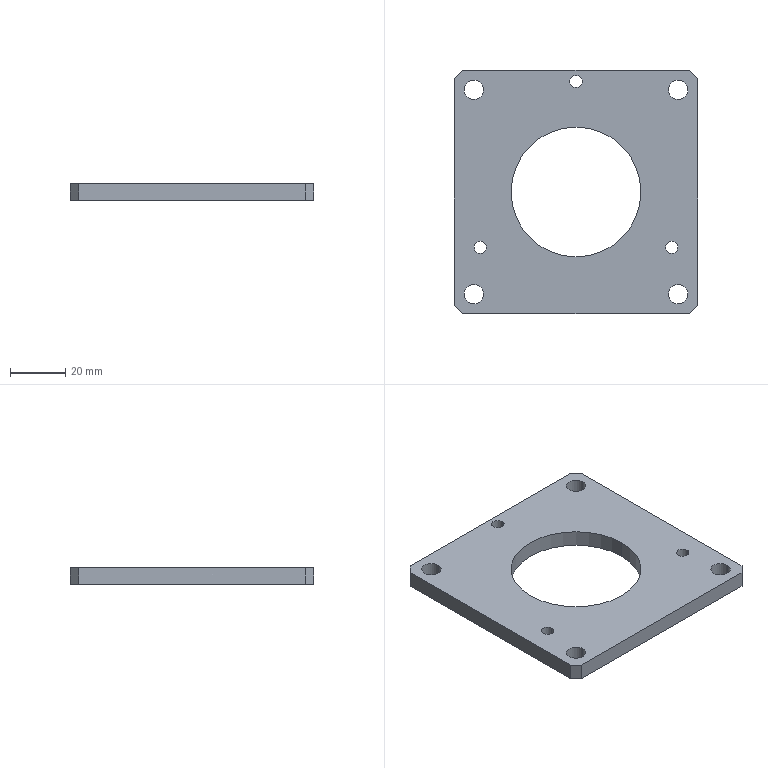Part | STEP file | MT-COMBO-119-S006 | 1 solid | 26 faces | box 88 x 88 x 6 mm | volume 34736 mm3 | cylinder 16 | plane 10 | commonest cylinder face diameters 7 x8 4.5 x6 47 x2
STEP:
#1=CARTESIAN_POINT('',(23.5,0.,6.));
#2=VERTEX_POINT('',#1);
#3=CARTESIAN_POINT('',(-23.5,0.,6.));
#4=VERTEX_POINT('',#3);
#5=CARTESIAN_POINT('',(0.,0.,6.));
#6=DIRECTION('',(0.,0.,1.));
#7=DIRECTION('',(-1.,0.,0.));
#8=AXIS2_PLACEMENT_3D('',#5,#6,#7);
#9=CIRCLE('',#8,23.5);
#10=EDGE_CURVE('',#2,#4,#9,.T.);
#11=ORIENTED_EDGE('',*,*,#10,.T.);
#12=CARTESIAN_POINT('',(-23.5,0.,0.));
#13=VERTEX_POINT('',#12);
#14=CARTESIAN_POINT('',(-23.5,0.,6.));
#15=DIRECTION('',(0.,0.,-1.));
#16=VECTOR('',#15,1000.);
#17=LINE('',#14,#16);
#18=EDGE_CURVE('',#4,#13,#17,.T.);
#19=ORIENTED_EDGE('',*,*,#18,.T.);
#20=CARTESIAN_POINT('',(23.5,0.,0.));
#21=VERTEX_POINT('',#20);
#22=CARTESIAN_POINT('',(0.,0.,0.));
#23=DIRECTION('',(0.,0.,1.));
#24=DIRECTION('',(-1.,0.,0.));
#25=AXIS2_PLACEMENT_3D('',#22,#23,#24);
#26=CIRCLE('',#25,23.5);
#27=EDGE_CURVE('',#21,#13,#26,.T.);
#28=ORIENTED_EDGE('',*,*,#27,.F.);
#29=CARTESIAN_POINT('',(23.5,0.,6.));
#30=DIRECTION('',(0.,0.,-1.));
#31=VECTOR('',#30,1000.);
#32=LINE('',#29,#31);
#33=EDGE_CURVE('',#2,#21,#32,.T.);
#34=ORIENTED_EDGE('',*,*,#33,.F.);
#35=EDGE_LOOP('',(#11,#19,#28,#34));
#36=FACE_OUTER_BOUND('',#35,.T.);
#37=CARTESIAN_POINT('',(0.,0.,6.));
#38=DIRECTION('',(0.,0.,-1.));
#39=DIRECTION('',(1.,0.,0.));
#40=AXIS2_PLACEMENT_3D('',#37,#38,#39);
#41=CYLINDRICAL_SURFACE('',#40,23.5);
#42=ADVANCED_FACE('',(#36),#41,.F.);
#43=CARTESIAN_POINT('',(-33.5,37.,6.));
#44=VERTEX_POINT('',#43);
#45=CARTESIAN_POINT('',(-40.5,37.,6.));
#46=VERTEX_POINT('',#45);
#47=CARTESIAN_POINT('',(-37.,37.,6.));
#48=DIRECTION('',(0.,0.,1.));
#49=DIRECTION('',(-1.,0.,0.));
#50=AXIS2_PLACEMENT_3D('',#47,#48,#49);
#51=CIRCLE('',#50,3.5);
#52=EDGE_CURVE('',#44,#46,#51,.T.);
#53=ORIENTED_EDGE('',*,*,#52,.T.);
#54=CARTESIAN_POINT('',(-40.5,37.,0.));
#55=VERTEX_POINT('',#54);
#56=CARTESIAN_POINT('',(-40.5,37.,6.));
#57=DIRECTION('',(0.,0.,-1.));
#58=VECTOR('',#57,1000.);
#59=LINE('',#56,#58);
#60=EDGE_CURVE('',#46,#55,#59,.T.);
#61=ORIENTED_EDGE('',*,*,#60,.T.);
#62=CARTESIAN_POINT('',(-33.5,37.,0.));
#63=VERTEX_POINT('',#62);
#64=CARTESIAN_POINT('',(-37.,37.,0.));
#65=DIRECTION('',(0.,0.,1.));
#66=DIRECTION('',(-1.,0.,0.));
#67=AXIS2_PLACEMENT_3D('',#64,#65,#66);
#68=CIRCLE('',#67,3.5);
#69=EDGE_CURVE('',#63,#55,#68,.T.);
#70=ORIENTED_EDGE('',*,*,#69,.F.);
#71=CARTESIAN_POINT('',(-33.5,37.,6.));
#72=DIRECTION('',(0.,0.,-1.));
#73=VECTOR('',#72,1000.);
#74=LINE('',#71,#73);
#75=EDGE_CURVE('',#44,#63,#74,.T.);
#76=ORIENTED_EDGE('',*,*,#75,.F.);
#77=EDGE_LOOP('',(#53,#61,#70,#76));
#78=FACE_OUTER_BOUND('',#77,.T.);
#79=CARTESIAN_POINT('',(-37.,37.,6.));
#80=DIRECTION('',(0.,0.,-1.));
#81=DIRECTION('',(1.,0.,0.));
#82=AXIS2_PLACEMENT_3D('',#79,#80,#81);
#83=CYLINDRICAL_SURFACE('',#82,3.5);
#84=ADVANCED_FACE('',(#78),#83,.F.);
#85=CARTESIAN_POINT('',(-33.5,-37.,6.));
#86=VERTEX_POINT('',#85);
#87=CARTESIAN_POINT('',(-40.5,-37.,6.));
#88=VERTEX_POINT('',#87);
#89=CARTESIAN_POINT('',(-37.,-37.,6.));
#90=DIRECTION('',(0.,0.,1.));
#91=DIRECTION('',(-1.,0.,0.));
#92=AXIS2_PLACEMENT_3D('',#89,#90,#91);
#93=CIRCLE('',#92,3.5);
#94=EDGE_CURVE('',#86,#88,#93,.T.);
#95=ORIENTED_EDGE('',*,*,#94,.T.);
#96=CARTESIAN_POINT('',(-40.5,-37.,0.));
#97=VERTEX_POINT('',#96);
#98=CARTESIAN_POINT('',(-40.5,-37.,6.));
#99=DIRECTION('',(0.,0.,-1.));
#100=VECTOR('',#99,1000.);
#101=LINE('',#98,#100);
#102=EDGE_CURVE('',#88,#97,#101,.T.);
#103=ORIENTED_EDGE('',*,*,#102,.T.);
#104=CARTESIAN_POINT('',(-33.5,-37.,0.));
#105=VERTEX_POINT('',#104);
#106=CARTESIAN_POINT('',(-37.,-37.,0.));
#107=DIRECTION('',(0.,0.,1.));
#108=DIRECTION('',(-1.,0.,0.));
#109=AXIS2_PLACEMENT_3D('',#106,#107,#108);
#110=CIRCLE('',#109,3.5);
#111=EDGE_CURVE('',#105,#97,#110,.T.);
#112=ORIENTED_EDGE('',*,*,#111,.F.);
#113=CARTESIAN_POINT('',(-33.5,-37.,6.));
#114=DIRECTION('',(0.,0.,-1.));
#115=VECTOR('',#114,1000.);
#116=LINE('',#113,#115);
#117=EDGE_CURVE('',#86,#105,#116,.T.);
#118=ORIENTED_EDGE('',*,*,#117,.F.);
#119=EDGE_LOOP('',(#95,#103,#112,#118));
#120=FACE_OUTER_BOUND('',#119,.T.);
#121=CARTESIAN_POINT('',(-37.,-37.,6.));
#122=DIRECTION('',(0.,0.,-1.));
#123=DIRECTION('',(1.,0.,0.));
#124=AXIS2_PLACEMENT_3D('',#121,#122,#123);
#125=CYLINDRICAL_SURFACE('',#124,3.5);
#126=ADVANCED_FACE('',(#120),#125,.F.);
#127=CARTESIAN_POINT('',(40.5,-37.,6.));
#128=VERTEX_POINT('',#127);
#129=CARTESIAN_POINT('',(33.5,-37.,6.));
#130=VERTEX_POINT('',#129);
#131=CARTESIAN_POINT('',(37.,-37.,6.));
#132=DIRECTION('',(0.,0.,1.));
#133=DIRECTION('',(-1.,0.,0.));
#134=AXIS2_PLACEMENT_3D('',#131,#132,#133);
#135=CIRCLE('',#134,3.5);
#136=EDGE_CURVE('',#128,#130,#135,.T.);
#137=ORIENTED_EDGE('',*,*,#136,.T.);
#138=CARTESIAN_POINT('',(33.5,-37.,0.));
#139=VERTEX_POINT('',#138);
#140=CARTESIAN_POINT('',(33.5,-37.,6.));
#141=DIRECTION('',(0.,0.,-1.));
#142=VECTOR('',#141,1000.);
#143=LINE('',#140,#142);
#144=EDGE_CURVE('',#130,#139,#143,.T.);
#145=ORIENTED_EDGE('',*,*,#144,.T.);
#146=CARTESIAN_POINT('',(40.5,-37.,0.));
#147=VERTEX_POINT('',#146);
#148=CARTESIAN_POINT('',(37.,-37.,0.));
#149=DIRECTION('',(0.,0.,1.));
#150=DIRECTION('',(-1.,0.,0.));
#151=AXIS2_PLACEMENT_3D('',#148,#149,#150);
#152=CIRCLE('',#151,3.5);
#153=EDGE_CURVE('',#147,#139,#152,.T.);
#154=ORIENTED_EDGE('',*,*,#153,.F.);
#155=CARTESIAN_POINT('',(40.5,-37.,6.));
#156=DIRECTION('',(0.,0.,-1.));
#157=VECTOR('',#156,1000.);
#158=LINE('',#155,#157);
#159=EDGE_CURVE('',#128,#147,#158,.T.);
#160=ORIENTED_EDGE('',*,*,#159,.F.);
#161=EDGE_LOOP('',(#137,#145,#154,#160));
#162=FACE_OUTER_BOUND('',#161,.T.);
#163=CARTESIAN_POINT('',(37.,-37.,6.));
#164=DIRECTION('',(0.,0.,-1.));
#165=DIRECTION('',(1.,0.,0.));
#166=AXIS2_PLACEMENT_3D('',#163,#164,#165);
#167=CYLINDRICAL_SURFACE('',#166,3.5);
#168=ADVANCED_FACE('',(#162),#167,.F.);
#169=CARTESIAN_POINT('',(40.5,37.,6.));
#170=VERTEX_POINT('',#169);
#171=CARTESIAN_POINT('',(33.5,37.,6.));
#172=VERTEX_POINT('',#171);
#173=CARTESIAN_POINT('',(37.,37.,6.));
#174=DIRECTION('',(0.,0.,1.));
#175=DIRECTION('',(-1.,0.,0.));
#176=AXIS2_PLACEMENT_3D('',#173,#174,#175);
#177=CIRCLE('',#176,3.5);
#178=EDGE_CURVE('',#170,#172,#177,.T.);
#179=ORIENTED_EDGE('',*,*,#178,.T.);
#180=CARTESIAN_POINT('',(33.5,37.,0.));
#181=VERTEX_POINT('',#180);
#182=CARTESIAN_POINT('',(33.5,37.,6.));
#183=DIRECTION('',(0.,0.,-1.));
#184=VECTOR('',#183,1000.);
#185=LINE('',#182,#184);
#186=EDGE_CURVE('',#172,#181,#185,.T.);
#187=ORIENTED_EDGE('',*,*,#186,.T.);
#188=CARTESIAN_POINT('',(40.5,37.,0.));
#189=VERTEX_POINT('',#188);
#190=CARTESIAN_POINT('',(37.,37.,0.));
#191=DIRECTION('',(0.,0.,1.));
#192=DIRECTION('',(-1.,0.,0.));
#193=AXIS2_PLACEMENT_3D('',#190,#191,#192);
#194=CIRCLE('',#193,3.5);
#195=EDGE_CURVE('',#189,#181,#194,.T.);
#196=ORIENTED_EDGE('',*,*,#195,.F.);
#197=CARTESIAN_POINT('',(40.5,37.,6.));
#198=DIRECTION('',(0.,0.,-1.));
#199=VECTOR('',#198,1000.);
#200=LINE('',#197,#199);
#201=EDGE_CURVE('',#170,#189,#200,.T.);
#202=ORIENTED_EDGE('',*,*,#201,.F.);
#203=EDGE_LOOP('',(#179,#187,#196,#202));
#204=FACE_OUTER_BOUND('',#203,.T.);
#205=CARTESIAN_POINT('',(37.,37.,6.));
#206=DIRECTION('',(0.,0.,-1.));
#207=DIRECTION('',(1.,0.,0.));
#208=AXIS2_PLACEMENT_3D('',#205,#206,#207);
#209=CYLINDRICAL_SURFACE('',#208,3.5);
#210=ADVANCED_FACE('',(#204),#209,.F.);
#211=CARTESIAN_POINT('',(2.25,40.,6.));
#212=VERTEX_POINT('',#211);
#213=CARTESIAN_POINT('',(-2.25,40.,6.));
#214=VERTEX_POINT('',#213);
#215=CARTESIAN_POINT('',(0.,40.,6.));
#216=DIRECTION('',(0.,0.,1.));
#217=DIRECTION('',(-1.,0.,0.));
#218=AXIS2_PLACEMENT_3D('',#215,#216,#217);
#219=CIRCLE('',#218,2.25);
#220=EDGE_CURVE('',#212,#214,#219,.T.);
#221=ORIENTED_EDGE('',*,*,#220,.T.);
#222=CARTESIAN_POINT('',(-2.25,40.,0.));
#223=VERTEX_POINT('',#222);
#224=CARTESIAN_POINT('',(-2.25,40.,6.));
#225=DIRECTION('',(0.,0.,-1.));
#226=VECTOR('',#225,1000.);
#227=LINE('',#224,#226);
#228=EDGE_CURVE('',#214,#223,#227,.T.);
#229=ORIENTED_EDGE('',*,*,#228,.T.);
#230=CARTESIAN_POINT('',(2.25,40.,0.));
#231=VERTEX_POINT('',#230);
#232=CARTESIAN_POINT('',(0.,40.,0.));
#233=DIRECTION('',(0.,0.,1.));
#234=DIRECTION('',(-1.,0.,0.));
#235=AXIS2_PLACEMENT_3D('',#232,#233,#234);
#236=CIRCLE('',#235,2.25);
#237=EDGE_CURVE('',#231,#223,#236,.T.);
#238=ORIENTED_EDGE('',*,*,#237,.F.);
#239=CARTESIAN_POINT('',(2.25,40.,6.));
#240=DIRECTION('',(0.,0.,-1.));
#241=VECTOR('',#240,1000.);
#242=LINE('',#239,#241);
#243=EDGE_CURVE('',#212,#231,#242,.T.);
#244=ORIENTED_EDGE('',*,*,#243,.F.);
#245=EDGE_LOOP('',(#221,#229,#238,#244));
#246=FACE_OUTER_BOUND('',#245,.T.);
#247=CARTESIAN_POINT('',(0.,40.,6.));
#248=DIRECTION('',(0.,0.,-1.));
#249=DIRECTION('',(1.,0.,0.));
#250=AXIS2_PLACEMENT_3D('',#247,#248,#249);
#251=CYLINDRICAL_SURFACE('',#250,2.25);
#252=ADVANCED_FACE('',(#246),#251,.F.);
#253=CARTESIAN_POINT('',(-32.391,-20.,6.));
#254=VERTEX_POINT('',#253);
#255=CARTESIAN_POINT('',(-36.891,-20.,6.));
#256=VERTEX_POINT('',#255);
#257=CARTESIAN_POINT('',(-34.641,-20.,6.));
#258=DIRECTION('',(0.,0.,1.));
#259=DIRECTION('',(-1.,0.,0.));
#260=AXIS2_PLACEMENT_3D('',#257,#258,#259);
#261=CIRCLE('',#260,2.25);
#262=EDGE_CURVE('',#254,#256,#261,.T.);
#263=ORIENTED_EDGE('',*,*,#262,.T.);
#264=CARTESIAN_POINT('',(-36.891,-20.,0.));
#265=VERTEX_POINT('',#264);
#266=CARTESIAN_POINT('',(-36.891,-20.,6.));
#267=DIRECTION('',(0.,0.,-1.));
#268=VECTOR('',#267,1000.);
#269=LINE('',#266,#268);
#270=EDGE_CURVE('',#256,#265,#269,.T.);
#271=ORIENTED_EDGE('',*,*,#270,.T.);
#272=CARTESIAN_POINT('',(-32.391,-20.,0.));
#273=VERTEX_POINT('',#272);
#274=CARTESIAN_POINT('',(-34.641,-20.,0.));
#275=DIRECTION('',(0.,0.,1.));
#276=DIRECTION('',(-1.,0.,0.));
#277=AXIS2_PLACEMENT_3D('',#274,#275,#276);
#278=CIRCLE('',#277,2.25);
#279=EDGE_CURVE('',#273,#265,#278,.T.);
#280=ORIENTED_EDGE('',*,*,#279,.F.);
#281=CARTESIAN_POINT('',(-32.391,-20.,6.));
#282=DIRECTION('',(0.,0.,-1.));
#283=VECTOR('',#282,1000.);
#284=LINE('',#281,#283);
#285=EDGE_CURVE('',#254,#273,#284,.T.);
#286=ORIENTED_EDGE('',*,*,#285,.F.);
#287=EDGE_LOOP('',(#263,#271,#280,#286));
#288=FACE_OUTER_BOUND('',#287,.T.);
#289=CARTESIAN_POINT('',(-34.641,-20.,6.));
#290=DIRECTION('',(0.,0.,-1.));
#291=DIRECTION('',(1.,0.,0.));
#292=AXIS2_PLACEMENT_3D('',#289,#290,#291);
#293=CYLINDRICAL_SURFACE('',#292,2.25);
#294=ADVANCED_FACE('',(#288),#293,.F.);
#295=CARTESIAN_POINT('',(36.891,-20.,6.));
#296=VERTEX_POINT('',#295);
#297=CARTESIAN_POINT('',(32.391,-20.,6.));
#298=VERTEX_POINT('',#297);
#299=CARTESIAN_POINT('',(34.641,-20.,6.));
#300=DIRECTION('',(0.,0.,1.));
#301=DIRECTION('',(-1.,0.,0.));
#302=AXIS2_PLACEMENT_3D('',#299,#300,#301);
#303=CIRCLE('',#302,2.25);
#304=EDGE_CURVE('',#296,#298,#303,.T.);
#305=ORIENTED_EDGE('',*,*,#304,.T.);
#306=CARTESIAN_POINT('',(32.391,-20.,0.));
#307=VERTEX_POINT('',#306);
#308=CARTESIAN_POINT('',(32.391,-20.,6.));
#309=DIRECTION('',(0.,0.,-1.));
#310=VECTOR('',#309,1000.);
#311=LINE('',#308,#310);
#312=EDGE_CURVE('',#298,#307,#311,.T.);
#313=ORIENTED_EDGE('',*,*,#312,.T.);
#314=CARTESIAN_POINT('',(36.891,-20.,0.));
#315=VERTEX_POINT('',#314);
#316=CARTESIAN_POINT('',(34.641,-20.,0.));
#317=DIRECTION('',(0.,0.,1.));
#318=DIRECTION('',(-1.,0.,0.));
#319=AXIS2_PLACEMENT_3D('',#316,#317,#318);
#320=CIRCLE('',#319,2.25);
#321=EDGE_CURVE('',#315,#307,#320,.T.);
#322=ORIENTED_EDGE('',*,*,#321,.F.);
#323=CARTESIAN_POINT('',(36.891,-20.,6.));
#324=DIRECTION('',(0.,0.,-1.));
#325=VECTOR('',#324,1000.);
#326=LINE('',#323,#325);
#327=EDGE_CURVE('',#296,#315,#326,.T.);
#328=ORIENTED_EDGE('',*,*,#327,.F.);
#329=EDGE_LOOP('',(#305,#313,#322,#328));
#330=FACE_OUTER_BOUND('',#329,.T.);
#331=CARTESIAN_POINT('',(34.641,-20.,6.));
#332=DIRECTION('',(0.,0.,-1.));
#333=DIRECTION('',(1.,0.,0.));
#334=AXIS2_PLACEMENT_3D('',#331,#332,#333);
#335=CYLINDRICAL_SURFACE('',#334,2.25);
#336=ADVANCED_FACE('',(#330),#335,.F.);
#337=CARTESIAN_POINT('',(41.,44.,6.));
#338=VERTEX_POINT('',#337);
#339=CARTESIAN_POINT('',(-41.,44.,6.));
#340=VERTEX_POINT('',#339);
#341=CARTESIAN_POINT('',(44.,44.,6.));
#342=DIRECTION('',(-1.,0.,0.));
#343=VECTOR('',#342,1000.);
#344=LINE('',#341,#343);
#345=EDGE_CURVE('',#338,#340,#344,.T.);
#346=ORIENTED_EDGE('',*,*,#345,.F.);
#347=CARTESIAN_POINT('',(41.,44.,0.));
#348=VERTEX_POINT('',#347);
#349=CARTESIAN_POINT('',(41.,44.,6.));
#350=DIRECTION('',(0.,0.,1.));
#351=VECTOR('',#350,1000.);
#352=LINE('',#349,#351);
#353=EDGE_CURVE('',#348,#338,#352,.T.);
#354=ORIENTED_EDGE('',*,*,#353,.F.);
#355=CARTESIAN_POINT('',(-41.,44.,0.));
#356=VERTEX_POINT('',#355);
#357=CARTESIAN_POINT('',(44.,44.,0.));
#358=DIRECTION('',(-1.,0.,0.));
#359=VECTOR('',#358,1000.);
#360=LINE('',#357,#359);
#361=EDGE_CURVE('',#348,#356,#360,.T.);
#362=ORIENTED_EDGE('',*,*,#361,.T.);
#363=CARTESIAN_POINT('',(-41.,44.,6.));
#364=DIRECTION('',(0.,0.,-1.));
#365=VECTOR('',#364,1000.);
#366=LINE('',#363,#365);
#367=EDGE_CURVE('',#340,#356,#366,.T.);
#368=ORIENTED_EDGE('',*,*,#367,.F.);
#369=EDGE_LOOP('',(#346,#354,#362,#368));
#370=FACE_OUTER_BOUND('',#369,.T.);
#371=CARTESIAN_POINT('',(44.,44.,6.));
#372=DIRECTION('',(0.,1.,0.));
#373=DIRECTION('',(0.,0.,-1.));
#374=AXIS2_PLACEMENT_3D('',#371,#372,#373);
#375=PLANE('',#374);
#376=ADVANCED_FACE('',(#370),#375,.T.);
#377=CARTESIAN_POINT('',(44.,-41.,0.));
#378=VERTEX_POINT('',#377);
#379=CARTESIAN_POINT('',(44.,41.,0.));
#380=VERTEX_POINT('',#379);
#381=CARTESIAN_POINT('',(44.,-44.,0.));
#382=DIRECTION('',(0.,1.,0.));
#383=VECTOR('',#382,1000.);
#384=LINE('',#381,#383);
#385=EDGE_CURVE('',#378,#380,#384,.T.);
#386=ORIENTED_EDGE('',*,*,#385,.T.);
#387=CARTESIAN_POINT('',(44.,41.,6.));
#388=VERTEX_POINT('',#387);
#389=CARTESIAN_POINT('',(44.,41.,6.));
#390=DIRECTION('',(0.,0.,-1.));
#391=VECTOR('',#390,1000.);
#392=LINE('',#389,#391);
#393=EDGE_CURVE('',#388,#380,#392,.T.);
#394=ORIENTED_EDGE('',*,*,#393,.F.);
#395=CARTESIAN_POINT('',(44.,-41.,6.));
#396=VERTEX_POINT('',#395);
#397=CARTESIAN_POINT('',(44.,-44.,6.));
#398=DIRECTION('',(0.,1.,0.));
#399=VECTOR('',#398,1000.);
#400=LINE('',#397,#399);
#401=EDGE_CURVE('',#396,#388,#400,.T.);
#402=ORIENTED_EDGE('',*,*,#401,.F.);
#403=CARTESIAN_POINT('',(44.,-41.,6.));
#404=DIRECTION('',(0.,0.,1.));
#405=VECTOR('',#404,1000.);
#406=LINE('',#403,#405);
#407=EDGE_CURVE('',#378,#396,#406,.T.);
#408=ORIENTED_EDGE('',*,*,#407,.F.);
#409=EDGE_LOOP('',(#386,#394,#402,#408));
#410=FACE_OUTER_BOUND('',#409,.T.);
#411=CARTESIAN_POINT('',(44.,-44.,6.));
#412=DIRECTION('',(1.,0.,0.));
#413=DIRECTION('',(0.,1.,0.));
#414=AXIS2_PLACEMENT_3D('',#411,#412,#413);
#415=PLANE('',#414);
#416=ADVANCED_FACE('',(#410),#415,.T.);
#417=CARTESIAN_POINT('',(-41.,-44.,0.));
#418=VERTEX_POINT('',#417);
#419=CARTESIAN_POINT('',(41.,-44.,0.));
#420=VERTEX_POINT('',#419);
#421=CARTESIAN_POINT('',(-44.,-44.,0.));
#422=DIRECTION('',(1.,0.,0.));
#423=VECTOR('',#422,1000.);
#424=LINE('',#421,#423);
#425=EDGE_CURVE('',#418,#420,#424,.T.);
#426=ORIENTED_EDGE('',*,*,#425,.T.);
#427=CARTESIAN_POINT('',(41.,-44.,6.));
#428=VERTEX_POINT('',#427);
#429=CARTESIAN_POINT('',(41.,-44.,6.));
#430=DIRECTION('',(0.,0.,-1.));
#431=VECTOR('',#430,1000.);
#432=LINE('',#429,#431);
#433=EDGE_CURVE('',#428,#420,#432,.T.);
#434=ORIENTED_EDGE('',*,*,#433,.F.);
#435=CARTESIAN_POINT('',(-41.,-44.,6.));
#436=VERTEX_POINT('',#435);
#437=CARTESIAN_POINT('',(-44.,-44.,6.));
#438=DIRECTION('',(1.,0.,0.));
#439=VECTOR('',#438,1000.);
#440=LINE('',#437,#439);
#441=EDGE_CURVE('',#436,#428,#440,.T.);
#442=ORIENTED_EDGE('',*,*,#441,.F.);
#443=CARTESIAN_POINT('',(-41.,-44.,6.));
#444=DIRECTION('',(0.,0.,1.));
#445=VECTOR('',#444,1000.);
#446=LINE('',#443,#445);
#447=EDGE_CURVE('',#418,#436,#446,.T.);
#448=ORIENTED_EDGE('',*,*,#447,.F.);
#449=EDGE_LOOP('',(#426,#434,#442,#448));
#450=FACE_OUTER_BOUND('',#449,.T.);
#451=CARTESIAN_POINT('',(-44.,-44.,6.));
#452=DIRECTION('',(0.,-1.,0.));
#453=DIRECTION('',(0.,0.,1.));
#454=AXIS2_PLACEMENT_3D('',#451,#452,#453);
#455=PLANE('',#454);
#456=ADVANCED_FACE('',(#450),#455,.T.);
#457=CARTESIAN_POINT('',(-44.,41.,6.));
#458=VERTEX_POINT('',#457);
#459=CARTESIAN_POINT('',(-44.,-41.,6.));
#460=VERTEX_POINT('',#459);
#461=CARTESIAN_POINT('',(-44.,44.,6.));
#462=DIRECTION('',(0.,-1.,0.));
#463=VECTOR('',#462,1000.);
#464=LINE('',#461,#463);
#465=EDGE_CURVE('',#458,#460,#464,.T.);
#466=ORIENTED_EDGE('',*,*,#465,.F.);
#467=CARTESIAN_POINT('',(-44.,41.,0.));
#468=VERTEX_POINT('',#467);
#469=CARTESIAN_POINT('',(-44.,41.,6.));
#470=DIRECTION('',(0.,0.,1.));
#471=VECTOR('',#470,1000.);
#472=LINE('',#469,#471);
#473=EDGE_CURVE('',#468,#458,#472,.T.);
#474=ORIENTED_EDGE('',*,*,#473,.F.);
#475=CARTESIAN_POINT('',(-44.,-41.,0.));
#476=VERTEX_POINT('',#475);
#477=CARTESIAN_POINT('',(-44.,44.,0.));
#478=DIRECTION('',(0.,-1.,0.));
#479=VECTOR('',#478,1000.);
#480=LINE('',#477,#479);
#481=EDGE_CURVE('',#468,#476,#480,.T.);
#482=ORIENTED_EDGE('',*,*,#481,.T.);
#483=CARTESIAN_POINT('',(-44.,-41.,6.));
#484=DIRECTION('',(0.,0.,-1.));
#485=VECTOR('',#484,1000.);
#486=LINE('',#483,#485);
#487=EDGE_CURVE('',#460,#476,#486,.T.);
#488=ORIENTED_EDGE('',*,*,#487,.F.);
#489=EDGE_LOOP('',(#466,#474,#482,#488));
#490=FACE_OUTER_BOUND('',#489,.T.);
#491=CARTESIAN_POINT('',(-44.,44.,6.));
#492=DIRECTION('',(-1.,0.,0.));
#493=DIRECTION('',(0.,-1.,0.));
#494=AXIS2_PLACEMENT_3D('',#491,#492,#493);
#495=PLANE('',#494);
#496=ADVANCED_FACE('',(#490),#495,.T.);
#497=ORIENTED_EDGE('',*,*,#10,.F.);
#498=CARTESIAN_POINT('',(0.,0.,6.));
#499=DIRECTION('',(0.,0.,1.));
#500=DIRECTION('',(-1.,0.,0.));
#501=AXIS2_PLACEMENT_3D('',#498,#499,#500);
#502=CIRCLE('',#501,23.5);
#503=EDGE_CURVE('',#4,#2,#502,.T.);
#504=ORIENTED_EDGE('',*,*,#503,.F.);
#505=EDGE_LOOP('',(#497,#504));
#506=FACE_BOUND('',#505,.T.);
#507=ORIENTED_EDGE('',*,*,#52,.F.);
#508=CARTESIAN_POINT('',(-37.,37.,6.));
#509=DIRECTION('',(0.,0.,1.));
#510=DIRECTION('',(-1.,0.,0.));
#511=AXIS2_PLACEMENT_3D('',#508,#509,#510);
#512=CIRCLE('',#511,3.5);
#513=EDGE_CURVE('',#46,#44,#512,.T.);
#514=ORIENTED_EDGE('',*,*,#513,.F.);
#515=EDGE_LOOP('',(#507,#514));
#516=FACE_BOUND('',#515,.T.);
#517=ORIENTED_EDGE('',*,*,#94,.F.);
#518=CARTESIAN_POINT('',(-37.,-37.,6.));
#519=DIRECTION('',(0.,0.,1.));
#520=DIRECTION('',(-1.,0.,0.));
#521=AXIS2_PLACEMENT_3D('',#518,#519,#520);
#522=CIRCLE('',#521,3.5);
#523=EDGE_CURVE('',#88,#86,#522,.T.);
#524=ORIENTED_EDGE('',*,*,#523,.F.);
#525=EDGE_LOOP('',(#517,#524));
#526=FACE_BOUND('',#525,.T.);
#527=ORIENTED_EDGE('',*,*,#136,.F.);
#528=CARTESIAN_POINT('',(37.,-37.,6.));
#529=DIRECTION('',(0.,0.,1.));
#530=DIRECTION('',(-1.,0.,0.));
#531=AXIS2_PLACEMENT_3D('',#528,#529,#530);
#532=CIRCLE('',#531,3.5);
#533=EDGE_CURVE('',#130,#128,#532,.T.);
#534=ORIENTED_EDGE('',*,*,#533,.F.);
#535=EDGE_LOOP('',(#527,#534));
#536=FACE_BOUND('',#535,.T.);
#537=ORIENTED_EDGE('',*,*,#178,.F.);
#538=CARTESIAN_POINT('',(37.,37.,6.));
#539=DIRECTION('',(0.,0.,1.));
#540=DIRECTION('',(-1.,0.,0.));
#541=AXIS2_PLACEMENT_3D('',#538,#539,#540);
#542=CIRCLE('',#541,3.5);
#543=EDGE_CURVE('',#172,#170,#542,.T.);
#544=ORIENTED_EDGE('',*,*,#543,.F.);
#545=EDGE_LOOP('',(#537,#544));
#546=FACE_BOUND('',#545,.T.);
#547=ORIENTED_EDGE('',*,*,#220,.F.);
#548=CARTESIAN_POINT('',(0.,40.,6.));
#549=DIRECTION('',(0.,0.,1.));
#550=DIRECTION('',(-1.,0.,0.));
#551=AXIS2_PLACEMENT_3D('',#548,#549,#550);
#552=CIRCLE('',#551,2.25);
#553=EDGE_CURVE('',#214,#212,#552,.T.);
#554=ORIENTED_EDGE('',*,*,#553,.F.);
#555=EDGE_LOOP('',(#547,#554));
#556=FACE_BOUND('',#555,.T.);
#557=ORIENTED_EDGE('',*,*,#262,.F.);
#558=CARTESIAN_POINT('',(-34.641,-20.,6.));
#559=DIRECTION('',(0.,0.,1.));
#560=DIRECTION('',(-1.,0.,0.));
#561=AXIS2_PLACEMENT_3D('',#558,#559,#560);
#562=CIRCLE('',#561,2.25);
#563=EDGE_CURVE('',#256,#254,#562,.T.);
#564=ORIENTED_EDGE('',*,*,#563,.F.);
#565=EDGE_LOOP('',(#557,#564));
#566=FACE_BOUND('',#565,.T.);
#567=ORIENTED_EDGE('',*,*,#304,.F.);
#568=CARTESIAN_POINT('',(34.641,-20.,6.));
#569=DIRECTION('',(0.,0.,1.));
#570=DIRECTION('',(-1.,0.,0.));
#571=AXIS2_PLACEMENT_3D('',#568,#569,#570);
#572=CIRCLE('',#571,2.25);
#573=EDGE_CURVE('',#298,#296,#572,.T.);
#574=ORIENTED_EDGE('',*,*,#573,.F.);
#575=EDGE_LOOP('',(#567,#574));
#576=FACE_BOUND('',#575,.T.);
#577=ORIENTED_EDGE('',*,*,#441,.T.);
#578=CARTESIAN_POINT('',(41.,-44.,6.));
#579=DIRECTION('',(-0.7071,-0.7071,0.));
#580=VECTOR('',#579,1000.);
#581=LINE('',#578,#580);
#582=EDGE_CURVE('',#396,#428,#581,.T.);
#583=ORIENTED_EDGE('',*,*,#582,.F.);
#584=ORIENTED_EDGE('',*,*,#401,.T.);
#585=CARTESIAN_POINT('',(44.,41.,6.));
#586=DIRECTION('',(0.7071,-0.7071,0.));
#587=VECTOR('',#586,1000.);
#588=LINE('',#585,#587);
#589=EDGE_CURVE('',#338,#388,#588,.T.);
#590=ORIENTED_EDGE('',*,*,#589,.F.);
#591=ORIENTED_EDGE('',*,*,#345,.T.);
#592=CARTESIAN_POINT('',(-41.,44.,6.));
#593=DIRECTION('',(0.7071,0.7071,0.));
#594=VECTOR('',#593,1000.);
#595=LINE('',#592,#594);
#596=EDGE_CURVE('',#458,#340,#595,.T.);
#597=ORIENTED_EDGE('',*,*,#596,.F.);
#598=ORIENTED_EDGE('',*,*,#465,.T.);
#599=CARTESIAN_POINT('',(-44.,-41.,6.));
#600=DIRECTION('',(-0.7071,0.7071,0.));
#601=VECTOR('',#600,1000.);
#602=LINE('',#599,#601);
#603=EDGE_CURVE('',#436,#460,#602,.T.);
#604=ORIENTED_EDGE('',*,*,#603,.F.);
#605=EDGE_LOOP('',(#577,#583,#584,#590,#591,#597,#598,#604));
#606=FACE_OUTER_BOUND('',#605,.T.);
#607=CARTESIAN_POINT('',(0.,0.,6.));
#608=DIRECTION('',(0.,0.,-1.));
#609=DIRECTION('',(1.,0.,0.));
#610=AXIS2_PLACEMENT_3D('',#607,#608,#609);
#611=PLANE('',#610);
#612=ADVANCED_FACE('',(#506,#516,#526,#536,#546,#556,#566,#576,#606),#611,.F.);
#613=ORIENTED_EDGE('',*,*,#27,.T.);
#614=CARTESIAN_POINT('',(0.,0.,0.));
#615=DIRECTION('',(0.,0.,1.));
#616=DIRECTION('',(-1.,0.,0.));
#617=AXIS2_PLACEMENT_3D('',#614,#615,#616);
#618=CIRCLE('',#617,23.5);
#619=EDGE_CURVE('',#13,#21,#618,.T.);
#620=ORIENTED_EDGE('',*,*,#619,.T.);
#621=EDGE_LOOP('',(#613,#620));
#622=FACE_BOUND('',#621,.T.);
#623=ORIENTED_EDGE('',*,*,#69,.T.);
#624=CARTESIAN_POINT('',(-37.,37.,0.));
#625=DIRECTION('',(0.,0.,1.));
#626=DIRECTION('',(-1.,0.,0.));
#627=AXIS2_PLACEMENT_3D('',#624,#625,#626);
#628=CIRCLE('',#627,3.5);
#629=EDGE_CURVE('',#55,#63,#628,.T.);
#630=ORIENTED_EDGE('',*,*,#629,.T.);
#631=EDGE_LOOP('',(#623,#630));
#632=FACE_BOUND('',#631,.T.);
#633=ORIENTED_EDGE('',*,*,#111,.T.);
#634=CARTESIAN_POINT('',(-37.,-37.,0.));
#635=DIRECTION('',(0.,0.,1.));
#636=DIRECTION('',(-1.,0.,0.));
#637=AXIS2_PLACEMENT_3D('',#634,#635,#636);
#638=CIRCLE('',#637,3.5);
#639=EDGE_CURVE('',#97,#105,#638,.T.);
#640=ORIENTED_EDGE('',*,*,#639,.T.);
#641=EDGE_LOOP('',(#633,#640));
#642=FACE_BOUND('',#641,.T.);
#643=ORIENTED_EDGE('',*,*,#153,.T.);
#644=CARTESIAN_POINT('',(37.,-37.,0.));
#645=DIRECTION('',(0.,0.,1.));
#646=DIRECTION('',(-1.,0.,0.));
#647=AXIS2_PLACEMENT_3D('',#644,#645,#646);
#648=CIRCLE('',#647,3.5);
#649=EDGE_CURVE('',#139,#147,#648,.T.);
#650=ORIENTED_EDGE('',*,*,#649,.T.);
#651=EDGE_LOOP('',(#643,#650));
#652=FACE_BOUND('',#651,.T.);
#653=ORIENTED_EDGE('',*,*,#195,.T.);
#654=CARTESIAN_POINT('',(37.,37.,0.));
#655=DIRECTION('',(0.,0.,1.));
#656=DIRECTION('',(-1.,0.,0.));
#657=AXIS2_PLACEMENT_3D('',#654,#655,#656);
#658=CIRCLE('',#657,3.5);
#659=EDGE_CURVE('',#181,#189,#658,.T.);
#660=ORIENTED_EDGE('',*,*,#659,.T.);
#661=EDGE_LOOP('',(#653,#660));
#662=FACE_BOUND('',#661,.T.);
#663=ORIENTED_EDGE('',*,*,#237,.T.);
#664=CARTESIAN_POINT('',(0.,40.,0.));
#665=DIRECTION('',(0.,0.,1.));
#666=DIRECTION('',(-1.,0.,0.));
#667=AXIS2_PLACEMENT_3D('',#664,#665,#666);
#668=CIRCLE('',#667,2.25);
#669=EDGE_CURVE('',#223,#231,#668,.T.);
#670=ORIENTED_EDGE('',*,*,#669,.T.);
#671=EDGE_LOOP('',(#663,#670));
#672=FACE_BOUND('',#671,.T.);
#673=ORIENTED_EDGE('',*,*,#279,.T.);
#674=CARTESIAN_POINT('',(-34.641,-20.,0.));
#675=DIRECTION('',(0.,0.,1.));
#676=DIRECTION('',(-1.,0.,0.));
#677=AXIS2_PLACEMENT_3D('',#674,#675,#676);
#678=CIRCLE('',#677,2.25);
#679=EDGE_CURVE('',#265,#273,#678,.T.);
#680=ORIENTED_EDGE('',*,*,#679,.T.);
#681=EDGE_LOOP('',(#673,#680));
#682=FACE_BOUND('',#681,.T.);
#683=ORIENTED_EDGE('',*,*,#321,.T.);
#684=CARTESIAN_POINT('',(34.641,-20.,0.));
#685=DIRECTION('',(0.,0.,1.));
#686=DIRECTION('',(-1.,0.,0.));
#687=AXIS2_PLACEMENT_3D('',#684,#685,#686);
#688=CIRCLE('',#687,2.25);
#689=EDGE_CURVE('',#307,#315,#688,.T.);
#690=ORIENTED_EDGE('',*,*,#689,.T.);
#691=EDGE_LOOP('',(#683,#690));
#692=FACE_BOUND('',#691,.T.);
#693=ORIENTED_EDGE('',*,*,#481,.F.);
#694=CARTESIAN_POINT('',(-42.5,42.5,0.));
#695=DIRECTION('',(-0.7071,-0.7071,0.));
#696=VECTOR('',#695,1000.);
#697=LINE('',#694,#696);
#698=EDGE_CURVE('',#356,#468,#697,.T.);
#699=ORIENTED_EDGE('',*,*,#698,.F.);
#700=ORIENTED_EDGE('',*,*,#361,.F.);
#701=CARTESIAN_POINT('',(42.5,42.5,0.));
#702=DIRECTION('',(-0.7071,0.7071,0.));
#703=VECTOR('',#702,1000.);
#704=LINE('',#701,#703);
#705=EDGE_CURVE('',#380,#348,#704,.T.);
#706=ORIENTED_EDGE('',*,*,#705,.F.);
#707=ORIENTED_EDGE('',*,*,#385,.F.);
#708=CARTESIAN_POINT('',(42.5,-42.5,0.));
#709=DIRECTION('',(0.7071,0.7071,0.));
#710=VECTOR('',#709,1000.);
#711=LINE('',#708,#710);
#712=EDGE_CURVE('',#420,#378,#711,.T.);
#713=ORIENTED_EDGE('',*,*,#712,.F.);
#714=ORIENTED_EDGE('',*,*,#425,.F.);
#715=CARTESIAN_POINT('',(-42.5,-42.5,0.));
#716=DIRECTION('',(0.7071,-0.7071,0.));
#717=VECTOR('',#716,1000.);
#718=LINE('',#715,#717);
#719=EDGE_CURVE('',#476,#418,#718,.T.);
#720=ORIENTED_EDGE('',*,*,#719,.F.);
#721=EDGE_LOOP('',(#693,#699,#700,#706,#707,#713,#714,#720));
#722=FACE_OUTER_BOUND('',#721,.T.);
#723=CARTESIAN_POINT('',(0.,0.,0.));
#724=DIRECTION('',(0.,0.,-1.));
#725=DIRECTION('',(1.,0.,0.));
#726=AXIS2_PLACEMENT_3D('',#723,#724,#725);
#727=PLANE('',#726);
#728=ADVANCED_FACE('',(#622,#632,#642,#652,#662,#672,#682,#692,#722),#727,.T.);
#729=ORIENTED_EDGE('',*,*,#312,.F.);
#730=ORIENTED_EDGE('',*,*,#573,.T.);
#731=ORIENTED_EDGE('',*,*,#327,.T.);
#732=ORIENTED_EDGE('',*,*,#689,.F.);
#733=EDGE_LOOP('',(#729,#730,#731,#732));
#734=FACE_OUTER_BOUND('',#733,.T.);
#735=CARTESIAN_POINT('',(34.641,-20.,6.));
#736=DIRECTION('',(0.,0.,-1.));
#737=DIRECTION('',(1.,0.,0.));
#738=AXIS2_PLACEMENT_3D('',#735,#736,#737);
#739=CYLINDRICAL_SURFACE('',#738,2.25);
#740=ADVANCED_FACE('',(#734),#739,.F.);
#741=ORIENTED_EDGE('',*,*,#270,.F.);
#742=ORIENTED_EDGE('',*,*,#563,.T.);
#743=ORIENTED_EDGE('',*,*,#285,.T.);
#744=ORIENTED_EDGE('',*,*,#679,.F.);
#745=EDGE_LOOP('',(#741,#742,#743,#744));
#746=FACE_OUTER_BOUND('',#745,.T.);
#747=CARTESIAN_POINT('',(-34.641,-20.,6.));
#748=DIRECTION('',(0.,0.,-1.));
#749=DIRECTION('',(1.,0.,0.));
#750=AXIS2_PLACEMENT_3D('',#747,#748,#749);
#751=CYLINDRICAL_SURFACE('',#750,2.25);
#752=ADVANCED_FACE('',(#746),#751,.F.);
#753=ORIENTED_EDGE('',*,*,#228,.F.);
#754=ORIENTED_EDGE('',*,*,#553,.T.);
#755=ORIENTED_EDGE('',*,*,#243,.T.);
#756=ORIENTED_EDGE('',*,*,#669,.F.);
#757=EDGE_LOOP('',(#753,#754,#755,#756));
#758=FACE_OUTER_BOUND('',#757,.T.);
#759=CARTESIAN_POINT('',(0.,40.,6.));
#760=DIRECTION('',(0.,0.,-1.));
#761=DIRECTION('',(1.,0.,0.));
#762=AXIS2_PLACEMENT_3D('',#759,#760,#761);
#763=CYLINDRICAL_SURFACE('',#762,2.25);
#764=ADVANCED_FACE('',(#758),#763,.F.);
#765=ORIENTED_EDGE('',*,*,#186,.F.);
#766=ORIENTED_EDGE('',*,*,#543,.T.);
#767=ORIENTED_EDGE('',*,*,#201,.T.);
#768=ORIENTED_EDGE('',*,*,#659,.F.);
#769=EDGE_LOOP('',(#765,#766,#767,#768));
#770=FACE_OUTER_BOUND('',#769,.T.);
#771=CARTESIAN_POINT('',(37.,37.,6.));
#772=DIRECTION('',(0.,0.,-1.));
#773=DIRECTION('',(1.,0.,0.));
#774=AXIS2_PLACEMENT_3D('',#771,#772,#773);
#775=CYLINDRICAL_SURFACE('',#774,3.5);
#776=ADVANCED_FACE('',(#770),#775,.F.);
#777=ORIENTED_EDGE('',*,*,#144,.F.);
#778=ORIENTED_EDGE('',*,*,#533,.T.);
#779=ORIENTED_EDGE('',*,*,#159,.T.);
#780=ORIENTED_EDGE('',*,*,#649,.F.);
#781=EDGE_LOOP('',(#777,#778,#779,#780));
#782=FACE_OUTER_BOUND('',#781,.T.);
#783=CARTESIAN_POINT('',(37.,-37.,6.));
#784=DIRECTION('',(0.,0.,-1.));
#785=DIRECTION('',(1.,0.,0.));
#786=AXIS2_PLACEMENT_3D('',#783,#784,#785);
#787=CYLINDRICAL_SURFACE('',#786,3.5);
#788=ADVANCED_FACE('',(#782),#787,.F.);
#789=ORIENTED_EDGE('',*,*,#102,.F.);
#790=ORIENTED_EDGE('',*,*,#523,.T.);
#791=ORIENTED_EDGE('',*,*,#117,.T.);
#792=ORIENTED_EDGE('',*,*,#639,.F.);
#793=EDGE_LOOP('',(#789,#790,#791,#792));
#794=FACE_OUTER_BOUND('',#793,.T.);
#795=CARTESIAN_POINT('',(-37.,-37.,6.));
#796=DIRECTION('',(0.,0.,-1.));
#797=DIRECTION('',(1.,0.,0.));
#798=AXIS2_PLACEMENT_3D('',#795,#796,#797);
#799=CYLINDRICAL_SURFACE('',#798,3.5);
#800=ADVANCED_FACE('',(#794),#799,.F.);
#801=ORIENTED_EDGE('',*,*,#60,.F.);
#802=ORIENTED_EDGE('',*,*,#513,.T.);
#803=ORIENTED_EDGE('',*,*,#75,.T.);
#804=ORIENTED_EDGE('',*,*,#629,.F.);
#805=EDGE_LOOP('',(#801,#802,#803,#804));
#806=FACE_OUTER_BOUND('',#805,.T.);
#807=CARTESIAN_POINT('',(-37.,37.,6.));
#808=DIRECTION('',(0.,0.,-1.));
#809=DIRECTION('',(1.,0.,0.));
#810=AXIS2_PLACEMENT_3D('',#807,#808,#809);
#811=CYLINDRICAL_SURFACE('',#810,3.5);
#812=ADVANCED_FACE('',(#806),#811,.F.);
#813=ORIENTED_EDGE('',*,*,#18,.F.);
#814=ORIENTED_EDGE('',*,*,#503,.T.);
#815=ORIENTED_EDGE('',*,*,#33,.T.);
#816=ORIENTED_EDGE('',*,*,#619,.F.);
#817=EDGE_LOOP('',(#813,#814,#815,#816));
#818=FACE_OUTER_BOUND('',#817,.T.);
#819=CARTESIAN_POINT('',(0.,0.,6.));
#820=DIRECTION('',(0.,0.,-1.));
#821=DIRECTION('',(1.,0.,0.));
#822=AXIS2_PLACEMENT_3D('',#819,#820,#821);
#823=CYLINDRICAL_SURFACE('',#822,23.5);
#824=ADVANCED_FACE('',(#818),#823,.F.);
#825=ORIENTED_EDGE('',*,*,#603,.T.);
#826=ORIENTED_EDGE('',*,*,#487,.T.);
#827=ORIENTED_EDGE('',*,*,#719,.T.);
#828=ORIENTED_EDGE('',*,*,#447,.T.);
#829=EDGE_LOOP('',(#825,#826,#827,#828));
#830=FACE_OUTER_BOUND('',#829,.T.);
#831=CARTESIAN_POINT('',(-44.,-41.,6.));
#832=DIRECTION('',(0.7071,0.7071,0.));
#833=DIRECTION('',(0.,0.,-1.));
#834=AXIS2_PLACEMENT_3D('',#831,#832,#833);
#835=PLANE('',#834);
#836=ADVANCED_FACE('',(#830),#835,.F.);
#837=ORIENTED_EDGE('',*,*,#582,.T.);
#838=ORIENTED_EDGE('',*,*,#433,.T.);
#839=ORIENTED_EDGE('',*,*,#712,.T.);
#840=ORIENTED_EDGE('',*,*,#407,.T.);
#841=EDGE_LOOP('',(#837,#838,#839,#840));
#842=FACE_OUTER_BOUND('',#841,.T.);
#843=CARTESIAN_POINT('',(41.,-44.,6.));
#844=DIRECTION('',(-0.7071,0.7071,0.));
#845=DIRECTION('',(0.,0.,-1.));
#846=AXIS2_PLACEMENT_3D('',#843,#844,#845);
#847=PLANE('',#846);
#848=ADVANCED_FACE('',(#842),#847,.F.);
#849=ORIENTED_EDGE('',*,*,#596,.T.);
#850=ORIENTED_EDGE('',*,*,#367,.T.);
#851=ORIENTED_EDGE('',*,*,#698,.T.);
#852=ORIENTED_EDGE('',*,*,#473,.T.);
#853=EDGE_LOOP('',(#849,#850,#851,#852));
#854=FACE_OUTER_BOUND('',#853,.T.);
#855=CARTESIAN_POINT('',(-41.,44.,6.));
#856=DIRECTION('',(0.7071,-0.7071,0.));
#857=DIRECTION('',(0.,0.,-1.));
#858=AXIS2_PLACEMENT_3D('',#855,#856,#857);
#859=PLANE('',#858);
#860=ADVANCED_FACE('',(#854),#859,.F.);
#861=ORIENTED_EDGE('',*,*,#589,.T.);
#862=ORIENTED_EDGE('',*,*,#393,.T.);
#863=ORIENTED_EDGE('',*,*,#705,.T.);
#864=ORIENTED_EDGE('',*,*,#353,.T.);
#865=EDGE_LOOP('',(#861,#862,#863,#864));
#866=FACE_OUTER_BOUND('',#865,.T.);
#867=CARTESIAN_POINT('',(44.,41.,6.));
#868=DIRECTION('',(-0.7071,-0.7071,0.));
#869=DIRECTION('',(0.,0.,-1.));
#870=AXIS2_PLACEMENT_3D('',#867,#868,#869);
#871=PLANE('',#870);
#872=ADVANCED_FACE('',(#866),#871,.F.);
#873=CLOSED_SHELL('',(#42,#84,#126,#168,#210,#252,#294,#336,#376,#416,#456,#496,#612,#728,#740,#752,#764,#776,#788,#800,#812,#824,#836,#848,#860,#872));
#874=MANIFOLD_SOLID_BREP('',#873);
#875=CARTESIAN_POINT('',(0.,0.,0.));
#876=DIRECTION('',(0.,0.,1.));
#877=DIRECTION('',(1.,0.,0.));
#878=AXIS2_PLACEMENT_3D('',#875,#876,#877);
#879=(LENGTH_UNIT()NAMED_UNIT(*)SI_UNIT(.MILLI.,.METRE.));
#880=UNCERTAINTY_MEASURE_WITH_UNIT(LENGTH_MEASURE(0.00001),#879,'','');
#881=(NAMED_UNIT(*)PLANE_ANGLE_UNIT()SI_UNIT($,.RADIAN.));
#882=(NAMED_UNIT(*)SI_UNIT($,.STERADIAN.)SOLID_ANGLE_UNIT());
#883=(GEOMETRIC_REPRESENTATION_CONTEXT(3)GLOBAL_UNCERTAINTY_ASSIGNED_CONTEXT((#880))GLOBAL_UNIT_ASSIGNED_CONTEXT((#879,#881,#882))REPRESENTATION_CONTEXT('',''));
#884=ADVANCED_BREP_SHAPE_REPRESENTATION('',(#874,#878),#883);